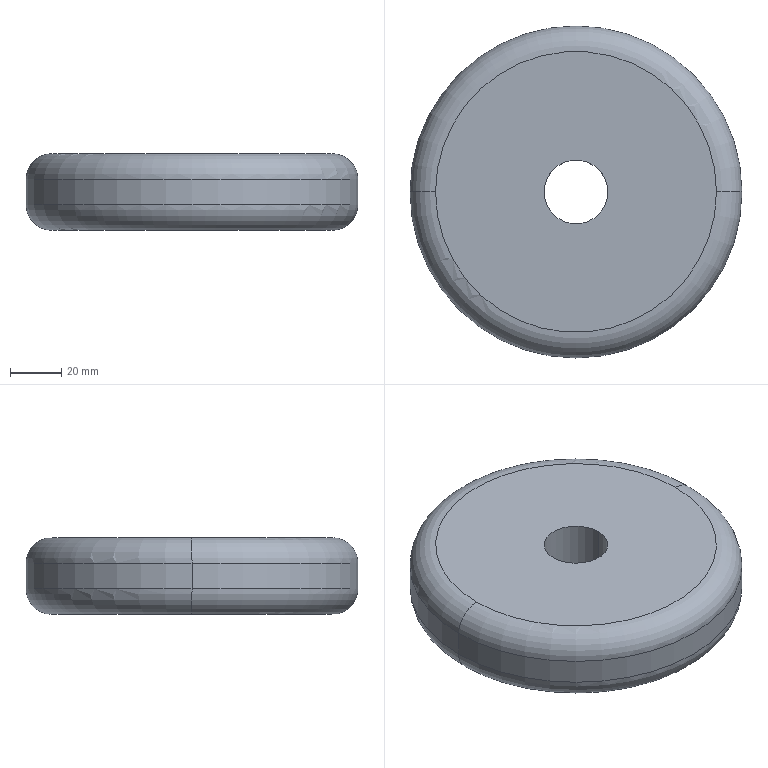Part | STEP file | 1 solid | 10 faces | box 130 x 130 x 30 mm | volume 366544 mm3 | torus 4 | cylinder 4 | plane 2 | commonest cylinder face diameters 25 x2 130 x2
STEP:
#1=CARTESIAN_POINT('',(0.,0.,0.));
#2=DIRECTION('',(0.,0.,1.));
#3=DIRECTION('',(1.,0.,0.));
#4=AXIS2_PLACEMENT_3D('',#1,#2,#3);
#5=CARTESIAN_POINT('',(-65.,0.,5.));
#6=VERTEX_POINT('',#5);
#7=CARTESIAN_POINT('',(65.,0.,5.));
#8=VERTEX_POINT('',#7);
#9=CARTESIAN_POINT('',(0.,0.,5.));
#10=DIRECTION('',(0.,0.,-1.));
#11=DIRECTION('',(1.,0.,0.));
#12=AXIS2_PLACEMENT_3D('',#9,#10,#11);
#13=CIRCLE('',#12,65.);
#14=CARTESIAN_POINT('',(0.,0.,5.));
#15=DIRECTION('',(0.,0.,1.));
#16=DIRECTION('',(1.,0.,0.));
#17=AXIS2_PLACEMENT_3D('',#14,#15,#16);
#18=TOROIDAL_SURFACE('',#17,55.,10.);
#19=CARTESIAN_POINT('',(6.283,0.));
#20=DIRECTION('',(-1.,0.));
#21=VECTOR('',#20,1.);
#22=LINE('',#19,#21);
#23=(GEOMETRIC_REPRESENTATION_CONTEXT(2)PARAMETRIC_REPRESENTATION_CONTEXT()REPRESENTATION_CONTEXT('',''));
#24=DEFINITIONAL_REPRESENTATION('',(#22),#23);
#25=PCURVE('',#18,#24);
#26=CARTESIAN_POINT('',(0.,0.,15.));
#27=DIRECTION('',(0.,0.,-1.));
#28=DIRECTION('',(-1.,0.,0.));
#29=AXIS2_PLACEMENT_3D('',#26,#27,#28);
#30=CYLINDRICAL_SURFACE('',#29,65.);
#31=CARTESIAN_POINT('',(-3.142,10.));
#32=DIRECTION('',(1.,0.));
#33=VECTOR('',#32,1.);
#34=LINE('',#31,#33);
#35=(GEOMETRIC_REPRESENTATION_CONTEXT(2)PARAMETRIC_REPRESENTATION_CONTEXT()REPRESENTATION_CONTEXT('',''));
#36=DEFINITIONAL_REPRESENTATION('',(#34),#35);
#37=PCURVE('',#30,#36);
#38=SURFACE_CURVE('',#13,(#25,#37),.PCURVE_S1.);
#39=EDGE_CURVE('',#6,#8,#38,.T.);
#40=ORIENTED_EDGE('',*,*,#39,.F.);
#41=CARTESIAN_POINT('',(-55.,0.,15.));
#42=VERTEX_POINT('',#41);
#43=CARTESIAN_POINT('',(-55.,0.,5.));
#44=DIRECTION('',(0.,1.,0.));
#45=DIRECTION('',(-1.,0.,0.));
#46=AXIS2_PLACEMENT_3D('',#43,#44,#45);
#47=CIRCLE('',#46,10.);
#48=CARTESIAN_POINT('',(3.142,0.));
#49=DIRECTION('',(0.,1.));
#50=VECTOR('',#49,1.);
#51=LINE('',#48,#50);
#52=(GEOMETRIC_REPRESENTATION_CONTEXT(2)PARAMETRIC_REPRESENTATION_CONTEXT()REPRESENTATION_CONTEXT('',''));
#53=DEFINITIONAL_REPRESENTATION('',(#51),#52);
#54=PCURVE('',#18,#53);
#55=CARTESIAN_POINT('',(0.,0.,5.));
#56=DIRECTION('',(0.,0.,1.));
#57=DIRECTION('',(1.,0.,0.));
#58=AXIS2_PLACEMENT_3D('',#55,#56,#57);
#59=TOROIDAL_SURFACE('',#58,55.,10.);
#60=CARTESIAN_POINT('',(3.142,0.));
#61=DIRECTION('',(0.,1.));
#62=VECTOR('',#61,1.);
#63=LINE('',#60,#62);
#64=(GEOMETRIC_REPRESENTATION_CONTEXT(2)PARAMETRIC_REPRESENTATION_CONTEXT()REPRESENTATION_CONTEXT('',''));
#65=DEFINITIONAL_REPRESENTATION('',(#63),#64);
#66=PCURVE('',#59,#65);
#67=SURFACE_CURVE('',#47,(#54,#66),.PCURVE_S1.);
#68=EDGE_CURVE('',#6,#42,#67,.T.);
#69=ORIENTED_EDGE('',*,*,#68,.T.);
#70=CARTESIAN_POINT('',(55.,0.,15.));
#71=VERTEX_POINT('',#70);
#72=CARTESIAN_POINT('',(0.,0.,15.));
#73=DIRECTION('',(0.,0.,1.));
#74=DIRECTION('',(1.,0.,0.));
#75=AXIS2_PLACEMENT_3D('',#72,#73,#74);
#76=CIRCLE('',#75,55.);
#77=CARTESIAN_POINT('',(0.,1.571));
#78=DIRECTION('',(1.,0.));
#79=VECTOR('',#78,1.);
#80=LINE('',#77,#79);
#81=(GEOMETRIC_REPRESENTATION_CONTEXT(2)PARAMETRIC_REPRESENTATION_CONTEXT()REPRESENTATION_CONTEXT('',''));
#82=DEFINITIONAL_REPRESENTATION('',(#80),#81);
#83=PCURVE('',#18,#82);
#84=CARTESIAN_POINT('',(0.,0.,15.));
#85=DIRECTION('',(0.,0.,1.));
#86=DIRECTION('',(1.,0.,0.));
#87=AXIS2_PLACEMENT_3D('',#84,#85,#86);
#88=PLANE('',#87);
#89=CARTESIAN_POINT('',(0.,0.));
#90=DIRECTION('',(1.,0.));
#91=AXIS2_PLACEMENT_2D('',#89,#90);
#92=CIRCLE('',#91,55.);
#93=(GEOMETRIC_REPRESENTATION_CONTEXT(2)PARAMETRIC_REPRESENTATION_CONTEXT()REPRESENTATION_CONTEXT('',''));
#94=DEFINITIONAL_REPRESENTATION('',(#92),#93);
#95=PCURVE('',#88,#94);
#96=SURFACE_CURVE('',#76,(#83,#95),.PCURVE_S1.);
#97=EDGE_CURVE('',#71,#42,#96,.T.);
#98=ORIENTED_EDGE('',*,*,#97,.F.);
#99=CARTESIAN_POINT('',(55.,0.,5.));
#100=DIRECTION('',(0.,-1.,0.));
#101=DIRECTION('',(0.,0.,-1.));
#102=AXIS2_PLACEMENT_3D('',#99,#100,#101);
#103=CIRCLE('',#102,10.);
#104=CARTESIAN_POINT('',(0.,-1.571));
#105=DIRECTION('',(0.,1.));
#106=VECTOR('',#105,1.);
#107=LINE('',#104,#106);
#108=(GEOMETRIC_REPRESENTATION_CONTEXT(2)PARAMETRIC_REPRESENTATION_CONTEXT()REPRESENTATION_CONTEXT('',''));
#109=DEFINITIONAL_REPRESENTATION('',(#107),#108);
#110=PCURVE('',#18,#109);
#111=CARTESIAN_POINT('',(6.283,-1.571));
#112=DIRECTION('',(0.,1.));
#113=VECTOR('',#112,1.);
#114=LINE('',#111,#113);
#115=(GEOMETRIC_REPRESENTATION_CONTEXT(2)PARAMETRIC_REPRESENTATION_CONTEXT()REPRESENTATION_CONTEXT('',''));
#116=DEFINITIONAL_REPRESENTATION('',(#114),#115);
#117=PCURVE('',#59,#116);
#118=SURFACE_CURVE('',#103,(#110,#117),.PCURVE_S1.);
#119=EDGE_CURVE('',#8,#71,#118,.T.);
#120=ORIENTED_EDGE('',*,*,#119,.F.);
#121=EDGE_LOOP('',(#40,#69,#98,#120));
#122=FACE_BOUND('',#121,.T.);
#123=ADVANCED_FACE('',(#122),#18,.T.);
#124=CARTESIAN_POINT('',(-55.,0.,-15.));
#125=VERTEX_POINT('',#124);
#126=CARTESIAN_POINT('',(55.,0.,-15.));
#127=VERTEX_POINT('',#126);
#128=CARTESIAN_POINT('',(0.,0.,-15.));
#129=DIRECTION('',(0.,0.,-1.));
#130=DIRECTION('',(1.,0.,0.));
#131=AXIS2_PLACEMENT_3D('',#128,#129,#130);
#132=CIRCLE('',#131,55.);
#133=CARTESIAN_POINT('',(0.,0.,-5.));
#134=DIRECTION('',(0.,0.,1.));
#135=DIRECTION('',(1.,0.,0.));
#136=AXIS2_PLACEMENT_3D('',#133,#134,#135);
#137=TOROIDAL_SURFACE('',#136,55.,10.);
#138=CARTESIAN_POINT('',(6.283,4.712));
#139=DIRECTION('',(-1.,0.));
#140=VECTOR('',#139,1.);
#141=LINE('',#138,#140);
#142=(GEOMETRIC_REPRESENTATION_CONTEXT(2)PARAMETRIC_REPRESENTATION_CONTEXT()REPRESENTATION_CONTEXT('',''));
#143=DEFINITIONAL_REPRESENTATION('',(#141),#142);
#144=PCURVE('',#137,#143);
#145=CARTESIAN_POINT('',(0.,0.,-15.));
#146=DIRECTION('',(0.,0.,1.));
#147=DIRECTION('',(1.,0.,0.));
#148=AXIS2_PLACEMENT_3D('',#145,#146,#147);
#149=PLANE('',#148);
#150=CARTESIAN_POINT('',(55.,0.));
#151=CARTESIAN_POINT('',(55.,-95.263));
#152=CARTESIAN_POINT('',(-27.5,-47.631));
#153=CARTESIAN_POINT('',(-110.,0.));
#154=CARTESIAN_POINT('',(-27.5,47.631));
#155=CARTESIAN_POINT('',(55.,95.263));
#156=CARTESIAN_POINT('',(55.,0.));
#157=(BOUNDED_CURVE()B_SPLINE_CURVE(2,(#150,#151,#152,#153,#154,#155,#156),.UNSPECIFIED.,.T.,.F.)B_SPLINE_CURVE_WITH_KNOTS((1,2,2,2,2,1),(-2.094,0.,2.094,4.189,6.283,8.378),.UNSPECIFIED.)CURVE()GEOMETRIC_REPRESENTATION_ITEM()RATIONAL_B_SPLINE_CURVE((1.,0.5,1.,0.5,1.,0.5,1.))REPRESENTATION_ITEM(''));
#158=(GEOMETRIC_REPRESENTATION_CONTEXT(2)PARAMETRIC_REPRESENTATION_CONTEXT()REPRESENTATION_CONTEXT('',''));
#159=DEFINITIONAL_REPRESENTATION('',(#157),#158);
#160=PCURVE('',#149,#159);
#161=SURFACE_CURVE('',#132,(#144,#160),.PCURVE_S1.);
#162=EDGE_CURVE('',#125,#127,#161,.T.);
#163=ORIENTED_EDGE('',*,*,#162,.F.);
#164=CARTESIAN_POINT('',(-65.,0.,-5.));
#165=VERTEX_POINT('',#164);
#166=CARTESIAN_POINT('',(-55.,0.,-5.));
#167=DIRECTION('',(0.,1.,0.));
#168=DIRECTION('',(-1.,0.,0.));
#169=AXIS2_PLACEMENT_3D('',#166,#167,#168);
#170=CIRCLE('',#169,10.);
#171=CARTESIAN_POINT('',(3.142,0.));
#172=DIRECTION('',(0.,1.));
#173=VECTOR('',#172,1.);
#174=LINE('',#171,#173);
#175=(GEOMETRIC_REPRESENTATION_CONTEXT(2)PARAMETRIC_REPRESENTATION_CONTEXT()REPRESENTATION_CONTEXT('',''));
#176=DEFINITIONAL_REPRESENTATION('',(#174),#175);
#177=PCURVE('',#137,#176);
#178=CARTESIAN_POINT('',(0.,0.,-5.));
#179=DIRECTION('',(0.,0.,1.));
#180=DIRECTION('',(1.,0.,0.));
#181=AXIS2_PLACEMENT_3D('',#178,#179,#180);
#182=TOROIDAL_SURFACE('',#181,55.,10.);
#183=CARTESIAN_POINT('',(3.142,0.));
#184=DIRECTION('',(0.,1.));
#185=VECTOR('',#184,1.);
#186=LINE('',#183,#185);
#187=(GEOMETRIC_REPRESENTATION_CONTEXT(2)PARAMETRIC_REPRESENTATION_CONTEXT()REPRESENTATION_CONTEXT('',''));
#188=DEFINITIONAL_REPRESENTATION('',(#186),#187);
#189=PCURVE('',#182,#188);
#190=SURFACE_CURVE('',#170,(#177,#189),.PCURVE_S1.);
#191=EDGE_CURVE('',#125,#165,#190,.T.);
#192=ORIENTED_EDGE('',*,*,#191,.T.);
#193=CARTESIAN_POINT('',(65.,0.,-5.));
#194=VERTEX_POINT('',#193);
#195=CARTESIAN_POINT('',(0.,0.,-5.));
#196=DIRECTION('',(0.,0.,1.));
#197=DIRECTION('',(1.,0.,0.));
#198=AXIS2_PLACEMENT_3D('',#195,#196,#197);
#199=CIRCLE('',#198,65.);
#200=CARTESIAN_POINT('',(0.,6.283));
#201=DIRECTION('',(1.,0.));
#202=VECTOR('',#201,1.);
#203=LINE('',#200,#202);
#204=(GEOMETRIC_REPRESENTATION_CONTEXT(2)PARAMETRIC_REPRESENTATION_CONTEXT()REPRESENTATION_CONTEXT('',''));
#205=DEFINITIONAL_REPRESENTATION('',(#203),#204);
#206=PCURVE('',#137,#205);
#207=CARTESIAN_POINT('',(3.142,20.));
#208=DIRECTION('',(-1.,0.));
#209=VECTOR('',#208,1.);
#210=LINE('',#207,#209);
#211=(GEOMETRIC_REPRESENTATION_CONTEXT(2)PARAMETRIC_REPRESENTATION_CONTEXT()REPRESENTATION_CONTEXT('',''));
#212=DEFINITIONAL_REPRESENTATION('',(#210),#211);
#213=PCURVE('',#30,#212);
#214=SURFACE_CURVE('',#199,(#206,#213),.PCURVE_S1.);
#215=EDGE_CURVE('',#194,#165,#214,.T.);
#216=ORIENTED_EDGE('',*,*,#215,.F.);
#217=CARTESIAN_POINT('',(55.,0.,-5.));
#218=DIRECTION('',(0.,-1.,0.));
#219=DIRECTION('',(0.,0.,-1.));
#220=AXIS2_PLACEMENT_3D('',#217,#218,#219);
#221=CIRCLE('',#220,10.);
#222=CARTESIAN_POINT('',(0.,4.712));
#223=DIRECTION('',(0.,1.));
#224=VECTOR('',#223,1.);
#225=LINE('',#222,#224);
#226=(GEOMETRIC_REPRESENTATION_CONTEXT(2)PARAMETRIC_REPRESENTATION_CONTEXT()REPRESENTATION_CONTEXT('',''));
#227=DEFINITIONAL_REPRESENTATION('',(#225),#226);
#228=PCURVE('',#137,#227);
#229=CARTESIAN_POINT('',(6.283,4.712));
#230=DIRECTION('',(0.,1.));
#231=VECTOR('',#230,1.);
#232=LINE('',#229,#231);
#233=(GEOMETRIC_REPRESENTATION_CONTEXT(2)PARAMETRIC_REPRESENTATION_CONTEXT()REPRESENTATION_CONTEXT('',''));
#234=DEFINITIONAL_REPRESENTATION('',(#232),#233);
#235=PCURVE('',#182,#234);
#236=SURFACE_CURVE('',#221,(#228,#235),.PCURVE_S1.);
#237=EDGE_CURVE('',#127,#194,#236,.T.);
#238=ORIENTED_EDGE('',*,*,#237,.F.);
#239=EDGE_LOOP('',(#163,#192,#216,#238));
#240=FACE_BOUND('',#239,.T.);
#241=ADVANCED_FACE('',(#240),#137,.T.);
#242=CARTESIAN_POINT('',(-12.5,0.,15.));
#243=VERTEX_POINT('',#242);
#244=CARTESIAN_POINT('',(-12.5,0.,-15.));
#245=VERTEX_POINT('',#244);
#246=CARTESIAN_POINT('',(-12.5,0.,15.));
#247=DIRECTION('',(0.,0.,-1.));
#248=VECTOR('',#247,1.);
#249=LINE('',#246,#248);
#250=CARTESIAN_POINT('',(0.,0.,15.));
#251=DIRECTION('',(0.,0.,-1.));
#252=DIRECTION('',(-1.,0.,0.));
#253=AXIS2_PLACEMENT_3D('',#250,#251,#252);
#254=CYLINDRICAL_SURFACE('',#253,12.5);
#255=CARTESIAN_POINT('',(6.283,0.));
#256=DIRECTION('',(0.,1.));
#257=VECTOR('',#256,1.);
#258=LINE('',#255,#257);
#259=(GEOMETRIC_REPRESENTATION_CONTEXT(2)PARAMETRIC_REPRESENTATION_CONTEXT()REPRESENTATION_CONTEXT('',''));
#260=DEFINITIONAL_REPRESENTATION('',(#258),#259);
#261=PCURVE('',#254,#260);
#262=CARTESIAN_POINT('',(0.,0.,15.));
#263=DIRECTION('',(0.,0.,-1.));
#264=DIRECTION('',(-1.,0.,0.));
#265=AXIS2_PLACEMENT_3D('',#262,#263,#264);
#266=CYLINDRICAL_SURFACE('',#265,12.5);
#267=CARTESIAN_POINT('',(0.,0.));
#268=DIRECTION('',(0.,1.));
#269=VECTOR('',#268,1.);
#270=LINE('',#267,#269);
#271=(GEOMETRIC_REPRESENTATION_CONTEXT(2)PARAMETRIC_REPRESENTATION_CONTEXT()REPRESENTATION_CONTEXT('',''));
#272=DEFINITIONAL_REPRESENTATION('',(#270),#271);
#273=PCURVE('',#266,#272);
#274=SURFACE_CURVE('',#249,(#261,#273),.PCURVE_S1.);
#275=EDGE_CURVE('',#243,#245,#274,.T.);
#276=ORIENTED_EDGE('',*,*,#275,.T.);
#277=CARTESIAN_POINT('',(12.5,0.,-15.));
#278=VERTEX_POINT('',#277);
#279=CARTESIAN_POINT('',(0.,0.,-15.));
#280=DIRECTION('',(0.,0.,1.));
#281=DIRECTION('',(1.,0.,0.));
#282=AXIS2_PLACEMENT_3D('',#279,#280,#281);
#283=CIRCLE('',#282,12.5);
#284=CARTESIAN_POINT('',(9.425,30.));
#285=DIRECTION('',(-1.,0.));
#286=VECTOR('',#285,1.);
#287=LINE('',#284,#286);
#288=(GEOMETRIC_REPRESENTATION_CONTEXT(2)PARAMETRIC_REPRESENTATION_CONTEXT()REPRESENTATION_CONTEXT('',''));
#289=DEFINITIONAL_REPRESENTATION('',(#287),#288);
#290=PCURVE('',#254,#289);
#291=CARTESIAN_POINT('',(0.,0.));
#292=DIRECTION('',(1.,0.));
#293=AXIS2_PLACEMENT_2D('',#291,#292);
#294=CIRCLE('',#293,12.5);
#295=(GEOMETRIC_REPRESENTATION_CONTEXT(2)PARAMETRIC_REPRESENTATION_CONTEXT()REPRESENTATION_CONTEXT('',''));
#296=DEFINITIONAL_REPRESENTATION('',(#294),#295);
#297=PCURVE('',#149,#296);
#298=SURFACE_CURVE('',#283,(#290,#297),.PCURVE_S1.);
#299=EDGE_CURVE('',#245,#278,#298,.T.);
#300=ORIENTED_EDGE('',*,*,#299,.T.);
#301=CARTESIAN_POINT('',(12.5,0.,15.));
#302=VERTEX_POINT('',#301);
#303=CARTESIAN_POINT('',(12.5,0.,15.));
#304=DIRECTION('',(0.,0.,-1.));
#305=VECTOR('',#304,1.);
#306=LINE('',#303,#305);
#307=CARTESIAN_POINT('',(3.142,0.));
#308=DIRECTION('',(0.,1.));
#309=VECTOR('',#308,1.);
#310=LINE('',#307,#309);
#311=(GEOMETRIC_REPRESENTATION_CONTEXT(2)PARAMETRIC_REPRESENTATION_CONTEXT()REPRESENTATION_CONTEXT('',''));
#312=DEFINITIONAL_REPRESENTATION('',(#310),#311);
#313=PCURVE('',#254,#312);
#314=CARTESIAN_POINT('',(3.142,0.));
#315=DIRECTION('',(0.,1.));
#316=VECTOR('',#315,1.);
#317=LINE('',#314,#316);
#318=(GEOMETRIC_REPRESENTATION_CONTEXT(2)PARAMETRIC_REPRESENTATION_CONTEXT()REPRESENTATION_CONTEXT('',''));
#319=DEFINITIONAL_REPRESENTATION('',(#317),#318);
#320=PCURVE('',#266,#319);
#321=SURFACE_CURVE('',#306,(#313,#320),.PCURVE_S1.);
#322=EDGE_CURVE('',#302,#278,#321,.T.);
#323=ORIENTED_EDGE('',*,*,#322,.F.);
#324=CARTESIAN_POINT('',(0.,0.,15.));
#325=DIRECTION('',(0.,0.,1.));
#326=DIRECTION('',(1.,0.,0.));
#327=AXIS2_PLACEMENT_3D('',#324,#325,#326);
#328=CIRCLE('',#327,12.5);
#329=CARTESIAN_POINT('',(9.425,0.));
#330=DIRECTION('',(-1.,0.));
#331=VECTOR('',#330,1.);
#332=LINE('',#329,#331);
#333=(GEOMETRIC_REPRESENTATION_CONTEXT(2)PARAMETRIC_REPRESENTATION_CONTEXT()REPRESENTATION_CONTEXT('',''));
#334=DEFINITIONAL_REPRESENTATION('',(#332),#333);
#335=PCURVE('',#254,#334);
#336=CARTESIAN_POINT('',(0.,0.));
#337=DIRECTION('',(1.,0.));
#338=AXIS2_PLACEMENT_2D('',#336,#337);
#339=CIRCLE('',#338,12.5);
#340=(GEOMETRIC_REPRESENTATION_CONTEXT(2)PARAMETRIC_REPRESENTATION_CONTEXT()REPRESENTATION_CONTEXT('',''));
#341=DEFINITIONAL_REPRESENTATION('',(#339),#340);
#342=PCURVE('',#88,#341);
#343=SURFACE_CURVE('',#328,(#335,#342),.PCURVE_S1.);
#344=EDGE_CURVE('',#243,#302,#343,.T.);
#345=ORIENTED_EDGE('',*,*,#344,.F.);
#346=EDGE_LOOP('',(#276,#300,#323,#345));
#347=FACE_BOUND('',#346,.F.);
#348=ADVANCED_FACE('',(#347),#254,.F.);
#349=ORIENTED_EDGE('',*,*,#39,.T.);
#350=CARTESIAN_POINT('',(65.,0.,15.));
#351=DIRECTION('',(0.,0.,-1.));
#352=VECTOR('',#351,1.);
#353=LINE('',#350,#352);
#354=CARTESIAN_POINT('',(3.142,0.));
#355=DIRECTION('',(0.,1.));
#356=VECTOR('',#355,1.);
#357=LINE('',#354,#356);
#358=(GEOMETRIC_REPRESENTATION_CONTEXT(2)PARAMETRIC_REPRESENTATION_CONTEXT()REPRESENTATION_CONTEXT('',''));
#359=DEFINITIONAL_REPRESENTATION('',(#357),#358);
#360=PCURVE('',#30,#359);
#361=CARTESIAN_POINT('',(0.,0.,15.));
#362=DIRECTION('',(0.,0.,-1.));
#363=DIRECTION('',(-1.,0.,0.));
#364=AXIS2_PLACEMENT_3D('',#361,#362,#363);
#365=CYLINDRICAL_SURFACE('',#364,65.);
#366=CARTESIAN_POINT('',(3.142,0.));
#367=DIRECTION('',(0.,1.));
#368=VECTOR('',#367,1.);
#369=LINE('',#366,#368);
#370=(GEOMETRIC_REPRESENTATION_CONTEXT(2)PARAMETRIC_REPRESENTATION_CONTEXT()REPRESENTATION_CONTEXT('',''));
#371=DEFINITIONAL_REPRESENTATION('',(#369),#370);
#372=PCURVE('',#365,#371);
#373=SURFACE_CURVE('',#353,(#360,#372),.PCURVE_S1.);
#374=EDGE_CURVE('',#8,#194,#373,.T.);
#375=ORIENTED_EDGE('',*,*,#374,.T.);
#376=ORIENTED_EDGE('',*,*,#215,.T.);
#377=CARTESIAN_POINT('',(-65.,0.,15.));
#378=DIRECTION('',(0.,0.,-1.));
#379=VECTOR('',#378,1.);
#380=LINE('',#377,#379);
#381=CARTESIAN_POINT('',(0.,0.));
#382=DIRECTION('',(0.,1.));
#383=VECTOR('',#382,1.);
#384=LINE('',#381,#383);
#385=(GEOMETRIC_REPRESENTATION_CONTEXT(2)PARAMETRIC_REPRESENTATION_CONTEXT()REPRESENTATION_CONTEXT('',''));
#386=DEFINITIONAL_REPRESENTATION('',(#384),#385);
#387=PCURVE('',#30,#386);
#388=CARTESIAN_POINT('',(6.283,0.));
#389=DIRECTION('',(0.,1.));
#390=VECTOR('',#389,1.);
#391=LINE('',#388,#390);
#392=(GEOMETRIC_REPRESENTATION_CONTEXT(2)PARAMETRIC_REPRESENTATION_CONTEXT()REPRESENTATION_CONTEXT('',''));
#393=DEFINITIONAL_REPRESENTATION('',(#391),#392);
#394=PCURVE('',#365,#393);
#395=SURFACE_CURVE('',#380,(#387,#394),.PCURVE_S1.);
#396=EDGE_CURVE('',#6,#165,#395,.T.);
#397=ORIENTED_EDGE('',*,*,#396,.F.);
#398=EDGE_LOOP('',(#349,#375,#376,#397));
#399=FACE_BOUND('',#398,.T.);
#400=ADVANCED_FACE('',(#399),#30,.T.);
#401=ORIENTED_EDGE('',*,*,#97,.T.);
#402=CARTESIAN_POINT('',(0.,0.,15.));
#403=DIRECTION('',(0.,0.,1.));
#404=DIRECTION('',(1.,0.,0.));
#405=AXIS2_PLACEMENT_3D('',#402,#403,#404);
#406=CIRCLE('',#405,55.);
#407=CARTESIAN_POINT('',(0.,0.));
#408=DIRECTION('',(1.,0.));
#409=AXIS2_PLACEMENT_2D('',#407,#408);
#410=CIRCLE('',#409,55.);
#411=(GEOMETRIC_REPRESENTATION_CONTEXT(2)PARAMETRIC_REPRESENTATION_CONTEXT()REPRESENTATION_CONTEXT('',''));
#412=DEFINITIONAL_REPRESENTATION('',(#410),#411);
#413=PCURVE('',#88,#412);
#414=CARTESIAN_POINT('',(0.,1.571));
#415=DIRECTION('',(1.,0.));
#416=VECTOR('',#415,1.);
#417=LINE('',#414,#416);
#418=(GEOMETRIC_REPRESENTATION_CONTEXT(2)PARAMETRIC_REPRESENTATION_CONTEXT()REPRESENTATION_CONTEXT('',''));
#419=DEFINITIONAL_REPRESENTATION('',(#417),#418);
#420=PCURVE('',#59,#419);
#421=SURFACE_CURVE('',#406,(#413,#420),.PCURVE_S1.);
#422=EDGE_CURVE('',#42,#71,#421,.T.);
#423=ORIENTED_EDGE('',*,*,#422,.T.);
#424=EDGE_LOOP('',(#401,#423));
#425=FACE_BOUND('',#424,.T.);
#426=ORIENTED_EDGE('',*,*,#344,.F.);
#427=CARTESIAN_POINT('',(0.,0.,15.));
#428=DIRECTION('',(0.,0.,1.));
#429=DIRECTION('',(1.,0.,0.));
#430=AXIS2_PLACEMENT_3D('',#427,#428,#429);
#431=CIRCLE('',#430,12.5);
#432=CARTESIAN_POINT('',(0.,0.));
#433=DIRECTION('',(1.,0.));
#434=AXIS2_PLACEMENT_2D('',#432,#433);
#435=CIRCLE('',#434,12.5);
#436=(GEOMETRIC_REPRESENTATION_CONTEXT(2)PARAMETRIC_REPRESENTATION_CONTEXT()REPRESENTATION_CONTEXT('',''));
#437=DEFINITIONAL_REPRESENTATION('',(#435),#436);
#438=PCURVE('',#88,#437);
#439=CARTESIAN_POINT('',(3.142,0.));
#440=DIRECTION('',(-1.,0.));
#441=VECTOR('',#440,1.);
#442=LINE('',#439,#441);
#443=(GEOMETRIC_REPRESENTATION_CONTEXT(2)PARAMETRIC_REPRESENTATION_CONTEXT()REPRESENTATION_CONTEXT('',''));
#444=DEFINITIONAL_REPRESENTATION('',(#442),#443);
#445=PCURVE('',#266,#444);
#446=SURFACE_CURVE('',#431,(#438,#445),.PCURVE_S1.);
#447=EDGE_CURVE('',#302,#243,#446,.T.);
#448=ORIENTED_EDGE('',*,*,#447,.F.);
#449=EDGE_LOOP('',(#426,#448));
#450=FACE_BOUND('',#449,.T.);
#451=ADVANCED_FACE('',(#425,#450),#88,.T.);
#452=CARTESIAN_POINT('',(0.,0.,-15.));
#453=DIRECTION('',(0.,0.,-1.));
#454=DIRECTION('',(1.,0.,0.));
#455=AXIS2_PLACEMENT_3D('',#452,#453,#454);
#456=CIRCLE('',#455,55.);
#457=CARTESIAN_POINT('',(55.,0.));
#458=CARTESIAN_POINT('',(55.,-95.263));
#459=CARTESIAN_POINT('',(-27.5,-47.631));
#460=CARTESIAN_POINT('',(-110.,0.));
#461=CARTESIAN_POINT('',(-27.5,47.631));
#462=CARTESIAN_POINT('',(55.,95.263));
#463=CARTESIAN_POINT('',(55.,0.));
#464=(BOUNDED_CURVE()B_SPLINE_CURVE(2,(#457,#458,#459,#460,#461,#462,#463),.UNSPECIFIED.,.T.,.F.)B_SPLINE_CURVE_WITH_KNOTS((1,2,2,2,2,1),(-2.094,0.,2.094,4.189,6.283,8.378),.UNSPECIFIED.)CURVE()GEOMETRIC_REPRESENTATION_ITEM()RATIONAL_B_SPLINE_CURVE((1.,0.5,1.,0.5,1.,0.5,1.))REPRESENTATION_ITEM(''));
#465=(GEOMETRIC_REPRESENTATION_CONTEXT(2)PARAMETRIC_REPRESENTATION_CONTEXT()REPRESENTATION_CONTEXT('',''));
#466=DEFINITIONAL_REPRESENTATION('',(#464),#465);
#467=PCURVE('',#149,#466);
#468=CARTESIAN_POINT('',(6.283,4.712));
#469=DIRECTION('',(-1.,0.));
#470=VECTOR('',#469,1.);
#471=LINE('',#468,#470);
#472=(GEOMETRIC_REPRESENTATION_CONTEXT(2)PARAMETRIC_REPRESENTATION_CONTEXT()REPRESENTATION_CONTEXT('',''));
#473=DEFINITIONAL_REPRESENTATION('',(#471),#472);
#474=PCURVE('',#182,#473);
#475=SURFACE_CURVE('',#456,(#467,#474),.PCURVE_S1.);
#476=EDGE_CURVE('',#127,#125,#475,.T.);
#477=ORIENTED_EDGE('',*,*,#476,.T.);
#478=ORIENTED_EDGE('',*,*,#162,.T.);
#479=EDGE_LOOP('',(#477,#478));
#480=FACE_BOUND('',#479,.T.);
#481=ORIENTED_EDGE('',*,*,#299,.T.);
#482=CARTESIAN_POINT('',(0.,0.,-15.));
#483=DIRECTION('',(0.,0.,1.));
#484=DIRECTION('',(1.,0.,0.));
#485=AXIS2_PLACEMENT_3D('',#482,#483,#484);
#486=CIRCLE('',#485,12.5);
#487=CARTESIAN_POINT('',(0.,0.));
#488=DIRECTION('',(1.,0.));
#489=AXIS2_PLACEMENT_2D('',#487,#488);
#490=CIRCLE('',#489,12.5);
#491=(GEOMETRIC_REPRESENTATION_CONTEXT(2)PARAMETRIC_REPRESENTATION_CONTEXT()REPRESENTATION_CONTEXT('',''));
#492=DEFINITIONAL_REPRESENTATION('',(#490),#491);
#493=PCURVE('',#149,#492);
#494=CARTESIAN_POINT('',(3.142,30.));
#495=DIRECTION('',(-1.,0.));
#496=VECTOR('',#495,1.);
#497=LINE('',#494,#496);
#498=(GEOMETRIC_REPRESENTATION_CONTEXT(2)PARAMETRIC_REPRESENTATION_CONTEXT()REPRESENTATION_CONTEXT('',''));
#499=DEFINITIONAL_REPRESENTATION('',(#497),#498);
#500=PCURVE('',#266,#499);
#501=SURFACE_CURVE('',#486,(#493,#500),.PCURVE_S1.);
#502=EDGE_CURVE('',#278,#245,#501,.T.);
#503=ORIENTED_EDGE('',*,*,#502,.T.);
#504=EDGE_LOOP('',(#481,#503));
#505=FACE_BOUND('',#504,.T.);
#506=ADVANCED_FACE('',(#480,#505),#149,.F.);
#507=ORIENTED_EDGE('',*,*,#374,.F.);
#508=CARTESIAN_POINT('',(0.,0.,5.));
#509=DIRECTION('',(0.,0.,-1.));
#510=DIRECTION('',(1.,0.,0.));
#511=AXIS2_PLACEMENT_3D('',#508,#509,#510);
#512=CIRCLE('',#511,65.);
#513=CARTESIAN_POINT('',(3.142,10.));
#514=DIRECTION('',(1.,0.));
#515=VECTOR('',#514,1.);
#516=LINE('',#513,#515);
#517=(GEOMETRIC_REPRESENTATION_CONTEXT(2)PARAMETRIC_REPRESENTATION_CONTEXT()REPRESENTATION_CONTEXT('',''));
#518=DEFINITIONAL_REPRESENTATION('',(#516),#517);
#519=PCURVE('',#365,#518);
#520=CARTESIAN_POINT('',(6.283,0.));
#521=DIRECTION('',(-1.,0.));
#522=VECTOR('',#521,1.);
#523=LINE('',#520,#522);
#524=(GEOMETRIC_REPRESENTATION_CONTEXT(2)PARAMETRIC_REPRESENTATION_CONTEXT()REPRESENTATION_CONTEXT('',''));
#525=DEFINITIONAL_REPRESENTATION('',(#523),#524);
#526=PCURVE('',#59,#525);
#527=SURFACE_CURVE('',#512,(#519,#526),.PCURVE_S1.);
#528=EDGE_CURVE('',#8,#6,#527,.T.);
#529=ORIENTED_EDGE('',*,*,#528,.T.);
#530=ORIENTED_EDGE('',*,*,#396,.T.);
#531=CARTESIAN_POINT('',(0.,0.,-5.));
#532=DIRECTION('',(0.,0.,1.));
#533=DIRECTION('',(1.,0.,0.));
#534=AXIS2_PLACEMENT_3D('',#531,#532,#533);
#535=CIRCLE('',#534,65.);
#536=CARTESIAN_POINT('',(9.425,20.));
#537=DIRECTION('',(-1.,0.));
#538=VECTOR('',#537,1.);
#539=LINE('',#536,#538);
#540=(GEOMETRIC_REPRESENTATION_CONTEXT(2)PARAMETRIC_REPRESENTATION_CONTEXT()REPRESENTATION_CONTEXT('',''));
#541=DEFINITIONAL_REPRESENTATION('',(#539),#540);
#542=PCURVE('',#365,#541);
#543=CARTESIAN_POINT('',(0.,6.283));
#544=DIRECTION('',(1.,0.));
#545=VECTOR('',#544,1.);
#546=LINE('',#543,#545);
#547=(GEOMETRIC_REPRESENTATION_CONTEXT(2)PARAMETRIC_REPRESENTATION_CONTEXT()REPRESENTATION_CONTEXT('',''));
#548=DEFINITIONAL_REPRESENTATION('',(#546),#547);
#549=PCURVE('',#182,#548);
#550=SURFACE_CURVE('',#535,(#542,#549),.PCURVE_S1.);
#551=EDGE_CURVE('',#165,#194,#550,.T.);
#552=ORIENTED_EDGE('',*,*,#551,.T.);
#553=EDGE_LOOP('',(#507,#529,#530,#552));
#554=FACE_BOUND('',#553,.T.);
#555=ADVANCED_FACE('',(#554),#365,.T.);
#556=ORIENTED_EDGE('',*,*,#502,.T.);
#557=ORIENTED_EDGE('',*,*,#275,.F.);
#558=ORIENTED_EDGE('',*,*,#447,.F.);
#559=ORIENTED_EDGE('',*,*,#322,.T.);
#560=EDGE_LOOP('',(#556,#557,#558,#559));
#561=FACE_BOUND('',#560,.F.);
#562=ADVANCED_FACE('',(#561),#266,.F.);
#563=ORIENTED_EDGE('',*,*,#191,.F.);
#564=ORIENTED_EDGE('',*,*,#476,.F.);
#565=ORIENTED_EDGE('',*,*,#237,.T.);
#566=ORIENTED_EDGE('',*,*,#551,.F.);
#567=EDGE_LOOP('',(#563,#564,#565,#566));
#568=FACE_BOUND('',#567,.T.);
#569=ADVANCED_FACE('',(#568),#182,.T.);
#570=ORIENTED_EDGE('',*,*,#68,.F.);
#571=ORIENTED_EDGE('',*,*,#528,.F.);
#572=ORIENTED_EDGE('',*,*,#119,.T.);
#573=ORIENTED_EDGE('',*,*,#422,.F.);
#574=EDGE_LOOP('',(#570,#571,#572,#573));
#575=FACE_BOUND('',#574,.T.);
#576=ADVANCED_FACE('',(#575),#59,.T.);
#577=CLOSED_SHELL('',(#123,#241,#348,#400,#451,#506,#555,#562,#569,#576));
#578=MANIFOLD_SOLID_BREP('',#577);
#579=(LENGTH_UNIT()NAMED_UNIT(*)SI_UNIT(.MILLI.,.METRE.));
#580=UNCERTAINTY_MEASURE_WITH_UNIT(LENGTH_MEASURE(0.0000001),#579,'','');
#581=(NAMED_UNIT(*)PLANE_ANGLE_UNIT()SI_UNIT($,.RADIAN.));
#582=(NAMED_UNIT(*)SI_UNIT($,.STERADIAN.)SOLID_ANGLE_UNIT());
#583=(GEOMETRIC_REPRESENTATION_CONTEXT(3)GLOBAL_UNCERTAINTY_ASSIGNED_CONTEXT((#580))GLOBAL_UNIT_ASSIGNED_CONTEXT((#579,#581,#582))REPRESENTATION_CONTEXT('',''));
#584=ADVANCED_BREP_SHAPE_REPRESENTATION('',(#4,#578),#583);